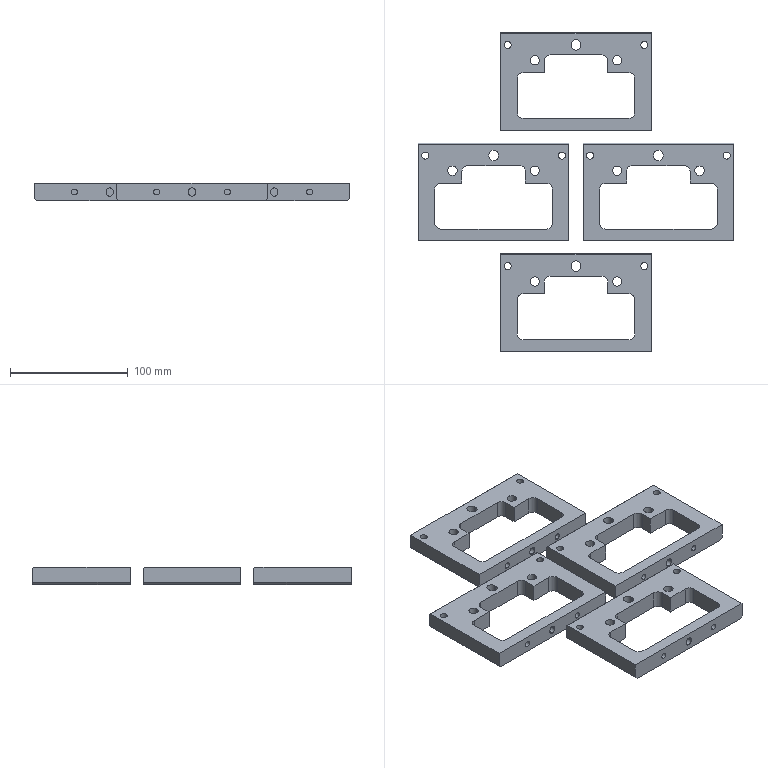NC program | NX | posted with a generic post | part box 268 x 271 x 15 mm
Lines 30 to 910 of 2286:
(ZLEVEL_PROFILE_COPY_COPY , TOOL : D4)
N52 T04 M6
N54 G54
N56 G17 G0 G90 X0.237 Y1.368 B0. C0. S9500 M3
N58 G43 Z30. H4
N60 Z1.5
N62 G94 G1 X0.139 Y1.399 Z1.495 F1000.
N64 X-0.131 Y1.401 Z1.48
N66 X-0.407 Y1.314 Z1.465
N68 X-0.642 Y1.145 Z1.45
N70 X-0.812 Y0.911 Z1.435
N72 X-0.9 Y0.635 Z1.42
N74 Y-0.612 Z1.354
N76 X-0.84 Y-0.851 Z1.342
N78 X-0.673 Y-1.113 Z1.325
N80 X-0.427 Y-1.304 Z1.309
N82 X-0.132 Y-1.4 Z1.293
N84 X0.179 Y-1.392 Z1.276
N86 X0.469 Y-1.28 Z1.26
N88 X0.677 Y-1.108 Z1.246
N90 X0.823 Y-0.888 Z1.232
N92 X0.9 Y-0.635 Z1.218
N94 Y0.635 Z1.152
N96 X0.813 Y0.909 Z1.137
N98 X0.645 Y1.142 Z1.122
N100 X0.412 Y1.311 Z1.106
N102 X0.139 Y1.399 Z1.091
N104 X-0.131 Y1.401 Z1.077
N106 X-0.407 Y1.314 Z1.062
N108 X-0.642 Y1.145 Z1.047
N110 X-0.812 Y0.911 Z1.032
N112 X-0.9 Y0.635 Z1.017
N114 Y-0.612 Z0.951
N116 X-0.84 Y-0.851 Z0.938
N118 X-0.673 Y-1.113 Z0.922
N120 X-0.427 Y-1.304 Z0.906
N122 X-0.132 Y-1.4 Z0.889
N124 X0.179 Y-1.392 Z0.873
N126 X0.469 Y-1.28 Z0.857
N128 X0.677 Y-1.108 Z0.843
N130 X0.823 Y-0.888 Z0.829
N132 X0.9 Y-0.635 Z0.815
N134 Y0.635 Z0.749
N136 X0.813 Y0.909 Z0.733
N138 X0.645 Y1.142 Z0.718
N140 X0.412 Y1.311 Z0.703
N142 X0.139 Y1.399 Z0.688
N144 X-0.131 Y1.401 Z0.674
N146 X-0.407 Y1.314 Z0.659
N148 X-0.642 Y1.145 Z0.644
N150 X-0.812 Y0.911 Z0.629
N152 X-0.9 Y0.635 Z0.613
N154 Y-0.612 Z0.548
N156 X-0.84 Y-0.851 Z0.535
N158 X-0.673 Y-1.113 Z0.519
N160 X-0.427 Y-1.304 Z0.503
N162 X-0.132 Y-1.4 Z0.486
N164 X0.179 Y-1.392 Z0.47
N166 X0.469 Y-1.28 Z0.454
N168 X0.677 Y-1.108 Z0.44
N170 X0.823 Y-0.888 Z0.426
N172 X0.9 Y-0.635 Z0.412
N174 Y0.635 Z0.345
N176 X0.813 Y0.909 Z0.33
N178 X0.645 Y1.142 Z0.315
N180 X0.412 Y1.311 Z0.3
N182 X0.139 Y1.399 Z0.285
N184 X-0.131 Y1.401 Z0.271
N186 X-0.407 Y1.314 Z0.256
N188 X-0.642 Y1.145 Z0.241
N190 X-0.812 Y0.911 Z0.225
N192 X-0.9 Y0.635 Z0.21
N194 Y-0.612 Z0.145
N196 X-0.84 Y-0.851 Z0.132
N198 X-0.673 Y-1.113 Z0.116
N200 X-0.427 Y-1.304 Z0.099
N202 X-0.132 Y-1.4 Z0.083
N204 X0.179 Y-1.392 Z0.067
N206 X0.469 Y-1.28 Z0.051
N208 X0.677 Y-1.108 Z0.036
N210 X0.823 Y-0.888 Z0.023
N212 X0.9 Y-0.635 Z0.009
N214 Y0.635 Z-0.058
N216 X0.813 Y0.909 Z-0.073
N218 X0.645 Y1.142 Z-0.088
N220 X0.412 Y1.311 Z-0.103
N222 X0.139 Y1.399 Z-0.118
N224 X-0.131 Y1.401 Z-0.132
N226 X-0.407 Y1.314 Z-0.147
N228 X-0.642 Y1.145 Z-0.163
N230 X-0.812 Y0.911 Z-0.178
N232 X-0.9 Y0.635 Z-0.193
N234 Y0.5 Z-0.2
N236 Y-0.5 F1200.
N238 G3 X0. Y-1.4 R0.9
N240 X0.9 Y-0.5 R0.9
N242 G1 Y0.5
N244 G3 X0. Y1.4 R0.9
N246 X-0.9 Y0.5 R0.9
N248 G1 Y-0.361 Z-0.23
N250 X-0.887 Y-0.589 Z-0.238
N252 X-0.881 Y-0.646 Z-0.24
N254 X-0.856 Y-0.754 Z-0.244
N256 X-0.838 Y-0.806 Z-0.246
N258 X-0.823 Y-0.843 Z-0.247
N260 X-0.791 Y-0.915 Z-0.25
N262 X-0.733 Y-1.009 Z-0.254
N264 X-0.7 Y-1.052 Z-0.256
N266 X-0.674 Y-1.083 Z-0.257
N268 X-0.62 Y-1.142 Z-0.26
N270 X-0.535 Y-1.215 Z-0.264
N272 X-0.456 Y-1.266 Z-0.267
N274 X-0.388 Y-1.304 Z-0.27
N276 X-0.285 Y-1.347 Z-0.274
N278 X-0.193 Y-1.37 Z-0.277
N280 X-0.116 Y-1.385 Z-0.28
N282 X-0.002 Y-1.394 Z-0.284
N284 X0.092 Y-1.387 Z-0.287
N286 X0.167 Y-1.376 Z-0.29
N288 X0.278 Y-1.349 Z-0.294
N290 X0.366 Y-1.313 Z-0.297
N292 X0.434 Y-1.28 Z-0.3
N294 X0.53 Y-1.219 Z-0.304
N296 X0.602 Y-1.158 Z-0.307
N298 X0.656 Y-1.104 Z-0.31
N300 X0.73 Y-1.015 Z-0.314
N302 X0.779 Y-0.934 Z-0.317
N304 X0.812 Y-0.868 Z-0.32
N306 X0.851 Y-0.775 Z-0.324
N308 X0.873 Y-0.683 Z-0.327
N310 X0.887 Y-0.595 Z-0.33
N312 X0.897 Y-0.452 Z-0.335
N314 X0.9 Y-0.309 Z-0.34
N316 Y0.265 Z-0.36
N318 Y0.409 Z-0.365
N320 X0.89 Y0.552 Z-0.37
N322 X0.873 Y0.681 Z-0.375
N324 X0.851 Y0.773 Z-0.378
N326 X0.828 Y0.828 Z-0.38
N328 X0.775 Y0.942 Z-0.384
N330 X0.725 Y1.023 Z-0.388
N332 X0.684 Y1.072 Z-0.39
N334 X0.584 Y1.173 Z-0.395
N336 X0.475 Y1.265 Z-0.4
N338 G3 X-0.9 Y0.5 R0.9
N340 G1 Y-0.361 Z-0.43
N342 X-0.887 Y-0.589 Z-0.438
N344 X-0.881 Y-0.646 Z-0.44
N346 X-0.856 Y-0.754 Z-0.444
N348 X-0.838 Y-0.806 Z-0.446
N350 X-0.823 Y-0.843 Z-0.447
N352 X-0.791 Y-0.915 Z-0.45
N354 X-0.733 Y-1.009 Z-0.454
N356 X-0.7 Y-1.052 Z-0.456
N358 X-0.674 Y-1.083 Z-0.457
N360 X-0.62 Y-1.142 Z-0.46
N362 X-0.535 Y-1.215 Z-0.464
N364 X-0.456 Y-1.266 Z-0.467
N366 X-0.388 Y-1.304 Z-0.47
N368 X-0.285 Y-1.347 Z-0.474
N370 X-0.193 Y-1.37 Z-0.477
N372 X-0.116 Y-1.385 Z-0.48
N374 X-0.002 Y-1.394 Z-0.484
N376 X0.092 Y-1.387 Z-0.487
N378 X0.167 Y-1.376 Z-0.49
N380 X0.278 Y-1.349 Z-0.494
N382 X0.366 Y-1.313 Z-0.497
N384 X0.434 Y-1.28 Z-0.5
N386 X0.53 Y-1.219 Z-0.504
N388 X0.602 Y-1.158 Z-0.507
N390 X0.656 Y-1.104 Z-0.51
N392 X0.73 Y-1.015 Z-0.514
N394 X0.779 Y-0.934 Z-0.517
N396 X0.812 Y-0.868 Z-0.52
N398 X0.85 Y-0.775 Z-0.524
N400 X0.873 Y-0.683 Z-0.527
N402 X0.887 Y-0.595 Z-0.53
N404 X0.897 Y-0.452 Z-0.535
N406 X0.9 Y-0.309 Z-0.54
N408 Y0.265 Z-0.56
N410 Y0.409 Z-0.565
N412 X0.89 Y0.552 Z-0.57
N414 X0.873 Y0.682 Z-0.575
N416 X0.851 Y0.773 Z-0.578
N418 X0.828 Y0.828 Z-0.58
N420 X0.775 Y0.942 Z-0.584
N422 X0.725 Y1.023 Z-0.588
N424 X0.684 Y1.072 Z-0.59
N426 X0.584 Y1.173 Z-0.595
N428 X0.475 Y1.265 Z-0.6
N430 G3 X-0.9 Y0.5 R0.9
N432 G1 Y-0.361 Z-0.63
N434 X-0.887 Y-0.589 Z-0.638
N436 X-0.881 Y-0.646 Z-0.64
N438 X-0.856 Y-0.754 Z-0.644
N440 X-0.838 Y-0.806 Z-0.646
N442 X-0.823 Y-0.843 Z-0.647
N444 X-0.791 Y-0.915 Z-0.65
N446 X-0.733 Y-1.009 Z-0.654
N448 X-0.701 Y-1.052 Z-0.656
N450 X-0.674 Y-1.083 Z-0.657
N452 X-0.62 Y-1.142 Z-0.66
N454 X-0.535 Y-1.215 Z-0.664
N456 X-0.456 Y-1.266 Z-0.667
N458 X-0.388 Y-1.304 Z-0.67
N460 X-0.285 Y-1.347 Z-0.674
N462 X-0.193 Y-1.37 Z-0.677
N464 X-0.116 Y-1.385 Z-0.68
N466 X-0.002 Y-1.394 Z-0.684
N468 X0.092 Y-1.387 Z-0.687
N470 X0.167 Y-1.376 Z-0.69
N472 X0.278 Y-1.349 Z-0.694
N474 X0.366 Y-1.313 Z-0.697
N476 X0.434 Y-1.28 Z-0.7
N478 X0.53 Y-1.219 Z-0.704
N480 X0.601 Y-1.158 Z-0.707
N482 X0.656 Y-1.104 Z-0.71
N484 X0.73 Y-1.015 Z-0.714
N486 X0.779 Y-0.934 Z-0.717
N488 X0.812 Y-0.868 Z-0.72
N490 X0.85 Y-0.775 Z-0.724
N492 X0.873 Y-0.683 Z-0.727
N494 X0.887 Y-0.595 Z-0.73
N496 X0.897 Y-0.452 Z-0.735
N498 X0.9 Y-0.309 Z-0.74
N500 Y0.265 Z-0.76
N502 Y0.409 Z-0.765
N504 X0.89 Y0.552 Z-0.77
N506 X0.873 Y0.682 Z-0.775
N508 X0.851 Y0.773 Z-0.778
N510 X0.828 Y0.828 Z-0.78
N512 X0.775 Y0.942 Z-0.784
N514 X0.725 Y1.022 Z-0.788
N516 X0.684 Y1.072 Z-0.79
N518 X0.584 Y1.173 Z-0.795
N520 X0.475 Y1.265 Z-0.8
N522 G3 X-0.9 Y0.5 R0.9
N524 G1 Y-0.361 Z-0.83
N526 X-0.887 Y-0.589 Z-0.838
N528 X-0.881 Y-0.646 Z-0.84
N530 X-0.856 Y-0.754 Z-0.844
N532 X-0.838 Y-0.806 Z-0.846
N534 X-0.823 Y-0.843 Z-0.847
N536 X-0.791 Y-0.915 Z-0.85
N538 X-0.733 Y-1.009 Z-0.854
N540 X-0.701 Y-1.052 Z-0.856
N542 X-0.675 Y-1.083 Z-0.857
N544 X-0.62 Y-1.142 Z-0.86
N546 X-0.535 Y-1.215 Z-0.864
N548 X-0.456 Y-1.266 Z-0.867
N550 X-0.388 Y-1.304 Z-0.87
N552 X-0.285 Y-1.347 Z-0.874
N554 X-0.193 Y-1.37 Z-0.877
N556 X-0.116 Y-1.385 Z-0.88
N558 X-0.003 Y-1.394 Z-0.884
N560 X0.092 Y-1.387 Z-0.887
N562 X0.167 Y-1.376 Z-0.89
N564 X0.278 Y-1.349 Z-0.894
N566 X0.365 Y-1.313 Z-0.897
N568 X0.434 Y-1.28 Z-0.9
N570 X0.53 Y-1.219 Z-0.904
N572 X0.601 Y-1.158 Z-0.907
N574 X0.656 Y-1.104 Z-0.91
N576 X0.729 Y-1.015 Z-0.914
N578 X0.779 Y-0.934 Z-0.917
N580 X0.812 Y-0.868 Z-0.92
N582 X0.85 Y-0.775 Z-0.924
N584 X0.873 Y-0.684 Z-0.927
N586 X0.887 Y-0.595 Z-0.93
N588 X0.897 Y-0.452 Z-0.935
N590 X0.9 Y-0.309 Z-0.94
N592 Y0.265 Z-0.96
N594 Y0.409 Z-0.965
N596 X0.89 Y0.552 Z-0.97
N598 X0.873 Y0.682 Z-0.975
N600 X0.851 Y0.773 Z-0.978
N602 X0.828 Y0.828 Z-0.98
N604 X0.775 Y0.942 Z-0.984
N606 X0.725 Y1.022 Z-0.988
N608 X0.684 Y1.072 Z-0.99
N610 X0.584 Y1.173 Z-0.995
N612 X0.475 Y1.265 Z-1.
N614 G3 X-0.9 Y0.5 R0.9
N616 G1 Y-0.361 Z-1.03
N618 X-0.887 Y-0.588 Z-1.038
N620 X-0.881 Y-0.646 Z-1.04
N622 X-0.856 Y-0.754 Z-1.044
N624 X-0.838 Y-0.806 Z-1.046
N626 X-0.823 Y-0.843 Z-1.047
N628 X-0.791 Y-0.915 Z-1.05
N630 X-0.733 Y-1.009 Z-1.054
N632 X-0.701 Y-1.052 Z-1.056
N634 X-0.675 Y-1.083 Z-1.057
N636 X-0.62 Y-1.142 Z-1.06
N638 X-0.535 Y-1.215 Z-1.064
N640 X-0.456 Y-1.266 Z-1.067
N642 X-0.388 Y-1.304 Z-1.07
N644 X-0.285 Y-1.347 Z-1.074
N646 X-0.193 Y-1.37 Z-1.077
N648 X-0.116 Y-1.385 Z-1.08
N650 X-0.003 Y-1.393 Z-1.084
N652 X0.092 Y-1.387 Z-1.087
N654 X0.167 Y-1.376 Z-1.09
N656 X0.278 Y-1.35 Z-1.094
N658 X0.365 Y-1.313 Z-1.097
N660 X0.434 Y-1.28 Z-1.1
N662 X0.53 Y-1.219 Z-1.104
N664 X0.602 Y-1.158 Z-1.107
N666 X0.656 Y-1.104 Z-1.11
N668 X0.73 Y-1.014 Z-1.114
N670 X0.78 Y-0.933 Z-1.117
N672 X0.812 Y-0.868 Z-1.12
N674 X0.85 Y-0.775 Z-1.124
N676 X0.873 Y-0.683 Z-1.127
N678 X0.887 Y-0.595 Z-1.13
N680 X0.897 Y-0.452 Z-1.135
N682 X0.9 Y-0.309 Z-1.14
N684 Y0.265 Z-1.16
N686 Y0.409 Z-1.165
N688 X0.89 Y0.552 Z-1.17
N690 X0.873 Y0.682 Z-1.175
N692 X0.851 Y0.773 Z-1.178
N694 X0.828 Y0.828 Z-1.18
N696 X0.775 Y0.942 Z-1.184
N698 X0.725 Y1.022 Z-1.188
N700 X0.684 Y1.071 Z-1.19
N702 X0.584 Y1.173 Z-1.195
N704 X0.475 Y1.265 Z-1.2
N706 G3 X-0.9 Y0.5 R0.9
N708 G1 Y-0.361 Z-1.23
N710 X-0.887 Y-0.588 Z-1.238
N712 X-0.881 Y-0.646 Z-1.24
N714 X-0.856 Y-0.754 Z-1.244
N716 X-0.838 Y-0.806 Z-1.246
N718 X-0.823 Y-0.842 Z-1.247
N720 X-0.791 Y-0.915 Z-1.25
N722 X-0.733 Y-1.008 Z-1.254
N724 X-0.701 Y-1.052 Z-1.256
N726 X-0.675 Y-1.082 Z-1.257
N728 X-0.62 Y-1.142 Z-1.26
N730 X-0.535 Y-1.215 Z-1.264
N732 X-0.456 Y-1.266 Z-1.267
N734 X-0.388 Y-1.304 Z-1.27
N736 X-0.285 Y-1.347 Z-1.274
N738 X-0.193 Y-1.37 Z-1.277
N740 X-0.116 Y-1.385 Z-1.28
N742 X-0.003 Y-1.393 Z-1.284
N744 X0.091 Y-1.387 Z-1.287
N746 X0.167 Y-1.376 Z-1.29
N748 X0.278 Y-1.35 Z-1.294
N750 X0.365 Y-1.313 Z-1.297
N752 X0.434 Y-1.28 Z-1.3
N754 X0.529 Y-1.219 Z-1.304
N756 X0.602 Y-1.158 Z-1.307
N758 X0.656 Y-1.104 Z-1.31
N760 X0.73 Y-1.014 Z-1.314
N762 X0.78 Y-0.933 Z-1.317
N764 X0.812 Y-0.868 Z-1.32
N766 X0.85 Y-0.775 Z-1.324
N768 X0.873 Y-0.683 Z-1.327
N770 X0.887 Y-0.595 Z-1.33
N772 X0.897 Y-0.452 Z-1.335
N774 X0.9 Y-0.309 Z-1.34
N776 Y0.265 Z-1.36
N778 Y0.409 Z-1.365
N780 X0.89 Y0.552 Z-1.37
N782 X0.873 Y0.682 Z-1.375
N784 X0.851 Y0.773 Z-1.378
N786 X0.828 Y0.828 Z-1.38
N788 X0.775 Y0.942 Z-1.384
N790 X0.725 Y1.022 Z-1.388
N792 X0.684 Y1.071 Z-1.39
N794 X0.584 Y1.173 Z-1.395
N796 X0.475 Y1.265 Z-1.4
N798 G3 X-0.9 Y0.5 R0.9
N800 G1 Y-0.361 Z-1.43
N802 X-0.887 Y-0.588 Z-1.438
N804 X-0.881 Y-0.646 Z-1.44
N806 X-0.856 Y-0.754 Z-1.444
N808 X-0.838 Y-0.806 Z-1.446
N810 X-0.823 Y-0.842 Z-1.447
N812 X-0.791 Y-0.915 Z-1.45
N814 X-0.733 Y-1.008 Z-1.454
N816 X-0.701 Y-1.052 Z-1.456
N818 X-0.675 Y-1.082 Z-1.457
N820 X-0.62 Y-1.142 Z-1.46
N822 X-0.535 Y-1.215 Z-1.464
N824 X-0.456 Y-1.266 Z-1.467
N826 X-0.388 Y-1.304 Z-1.47
N828 X-0.285 Y-1.347 Z-1.474
N830 X-0.193 Y-1.37 Z-1.477
N832 X-0.116 Y-1.385 Z-1.48
N834 X-0.003 Y-1.393 Z-1.484
N836 X0.091 Y-1.387 Z-1.487
N838 X0.167 Y-1.376 Z-1.49
N840 X0.278 Y-1.35 Z-1.494
N842 X0.365 Y-1.313 Z-1.497
N844 X0.434 Y-1.28 Z-1.5
N846 X0.531 Y-1.218 Z-1.504
N848 X0.603 Y-1.158 Z-1.507
N850 X0.656 Y-1.104 Z-1.51
N852 X0.73 Y-1.013 Z-1.514
N854 X0.78 Y-0.933 Z-1.517
N856 X0.812 Y-0.868 Z-1.52
N858 X0.85 Y-0.775 Z-1.524
N860 X0.873 Y-0.683 Z-1.527
N862 X0.887 Y-0.595 Z-1.53
N864 X0.897 Y-0.452 Z-1.535
N866 X0.9 Y-0.309 Z-1.54
N868 Y0.265 Z-1.56
N870 Y0.409 Z-1.565
N872 X0.889 Y0.552 Z-1.57
N874 X0.873 Y0.682 Z-1.575
N876 X0.851 Y0.773 Z-1.578
N878 X0.828 Y0.828 Z-1.58
N880 X0.775 Y0.942 Z-1.584
N882 X0.725 Y1.022 Z-1.588
N884 X0.684 Y1.071 Z-1.59
N886 X0.584 Y1.173 Z-1.595
N888 X0.475 Y1.265 Z-1.6
N890 G3 X-0.9 Y0.5 R0.9
N892 G1 Y-0.361 Z-1.63
N894 X-0.887 Y-0.588 Z-1.638
N896 X-0.881 Y-0.646 Z-1.64
N898 X-0.856 Y-0.754 Z-1.644
N900 X-0.838 Y-0.806 Z-1.646
N902 X-0.823 Y-0.842 Z-1.647
N904 X-0.791 Y-0.915 Z-1.65
N906 X-0.733 Y-1.008 Z-1.654
N908 X-0.701 Y-1.052 Z-1.656
N910 X-0.675 Y-1.082 Z-1.657
N912 X-0.62 Y-1.142 Z-1.66
N914 X-0.535 Y-1.215 Z-1.664
N916 X-0.456 Y-1.266 Z-1.667
N918 X-0.388 Y-1.304 Z-1.67
N920 X-0.285 Y-1.347 Z-1.674
N922 X-0.193 Y-1.37 Z-1.677
N924 X-0.116 Y-1.385 Z-1.68
N926 X-0.003 Y-1.394 Z-1.684
N928 X0.091 Y-1.386 Z-1.687
N930 X0.167 Y-1.376 Z-1.69
N932 X0.278 Y-1.35 Z-1.694
N934 X0.365 Y-1.313 Z-1.697
N936 X0.434 Y-1.28 Z-1.7
N938 X0.53 Y-1.219 Z-1.704
N940 X0.603 Y-1.158 Z-1.707
N942 X0.656 Y-1.104 Z-1.71
N944 X0.73 Y-1.013 Z-1.714
N946 X0.78 Y-0.933 Z-1.717
N948 X0.812 Y-0.868 Z-1.72
N950 X0.85 Y-0.775 Z-1.724
N952 X0.872 Y-0.683 Z-1.727
N954 X0.887 Y-0.595 Z-1.73
N956 X0.897 Y-0.452 Z-1.735
N958 X0.9 Y-0.309 Z-1.74
N960 Y0.265 Z-1.76
N962 Y0.409 Z-1.765
N964 X0.889 Y0.552 Z-1.77
N966 X0.873 Y0.682 Z-1.775
N968 X0.851 Y0.773 Z-1.778
N970 X0.828 Y0.828 Z-1.78
N972 X0.775 Y0.942 Z-1.784
N974 X0.725 Y1.022 Z-1.788
N976 X0.684 Y1.071 Z-1.79
N978 X0.584 Y1.173 Z-1.795
N980 X0.475 Y1.265 Z-1.8
N982 G3 X-0.9 Y0.5 R0.9
N984 G1 Y-0.361 Z-1.83
N986 X-0.887 Y-0.588 Z-1.838
N988 X-0.881 Y-0.646 Z-1.84
N990 X-0.856 Y-0.754 Z-1.844
N992 X-0.838 Y-0.806 Z-1.846
N994 X-0.823 Y-0.842 Z-1.847
N996 X-0.791 Y-0.915 Z-1.85
N998 X-0.733 Y-1.008 Z-1.854
N1000 X-0.701 Y-1.052 Z-1.856
N1002 X-0.675 Y-1.082 Z-1.857
N1004 X-0.62 Y-1.142 Z-1.86
N1006 X-0.535 Y-1.215 Z-1.864
N1008 X-0.456 Y-1.266 Z-1.867
N1010 X-0.388 Y-1.304 Z-1.87
N1012 X-0.285 Y-1.347 Z-1.874
N1014 X-0.194 Y-1.37 Z-1.877
N1016 X-0.116 Y-1.385 Z-1.88
N1018 X-0.003 Y-1.394 Z-1.884
N1020 X0.091 Y-1.386 Z-1.887
N1022 X0.167 Y-1.376 Z-1.89
N1024 X0.278 Y-1.35 Z-1.894
N1026 X0.365 Y-1.313 Z-1.897
N1028 X0.434 Y-1.28 Z-1.9
N1030 X0.531 Y-1.219 Z-1.904
N1032 X0.602 Y-1.158 Z-1.907
N1034 X0.656 Y-1.104 Z-1.91
N1036 X0.73 Y-1.013 Z-1.914
N1038 X0.78 Y-0.933 Z-1.917
N1040 X0.812 Y-0.868 Z-1.92
N1042 X0.85 Y-0.775 Z-1.924
N1044 X0.872 Y-0.683 Z-1.927
N1046 X0.887 Y-0.595 Z-1.93
N1048 X0.897 Y-0.452 Z-1.935
N1050 X0.9 Y-0.309 Z-1.94
N1052 Y0.265 Z-1.96
N1054 Y0.409 Z-1.965
N1056 X0.889 Y0.552 Z-1.97
N1058 X0.873 Y0.682 Z-1.975
N1060 X0.851 Y0.773 Z-1.978
N1062 X0.828 Y0.828 Z-1.98
N1064 X0.775 Y0.942 Z-1.984
N1066 X0.725 Y1.022 Z-1.988
N1068 X0.684 Y1.071 Z-1.99
N1070 X0.584 Y1.173 Z-1.995
N1072 X0.475 Y1.265 Z-2.
N1074 G3 X-0.9 Y0.5 R0.9
N1076 G1 Y-0.361 Z-2.03
N1078 X-0.887 Y-0.588 Z-2.038
N1080 X-0.881 Y-0.646 Z-2.04
N1082 X-0.856 Y-0.754 Z-2.044
N1084 X-0.838 Y-0.806 Z-2.046
N1086 X-0.823 Y-0.842 Z-2.047
N1088 X-0.791 Y-0.915 Z-2.05
N1090 X-0.734 Y-1.009 Z-2.054
N1092 X-0.701 Y-1.052 Z-2.056
N1094 X-0.675 Y-1.082 Z-2.057
N1096 X-0.62 Y-1.142 Z-2.06
N1098 X-0.535 Y-1.215 Z-2.064
N1100 X-0.456 Y-1.266 Z-2.067
N1102 X-0.388 Y-1.304 Z-2.07
N1104 X-0.285 Y-1.346 Z-2.074
N1106 X-0.194 Y-1.37 Z-2.077
N1108 X-0.116 Y-1.385 Z-2.08
N1110 X-0.003 Y-1.394 Z-2.084
N1112 X0.091 Y-1.386 Z-2.087
N1114 X0.167 Y-1.376 Z-2.09
N1116 X0.278 Y-1.35 Z-2.094
N1118 X0.365 Y-1.313 Z-2.097
N1120 X0.434 Y-1.28 Z-2.1
N1122 X0.531 Y-1.219 Z-2.104
N1124 X0.602 Y-1.158 Z-2.107
N1126 X0.656 Y-1.104 Z-2.11
N1128 X0.731 Y-1.014 Z-2.114
N1130 X0.78 Y-0.933 Z-2.117
N1132 X0.812 Y-0.868 Z-2.12
N1134 X0.85 Y-0.775 Z-2.124
N1136 X0.872 Y-0.683 Z-2.127
N1138 X0.886 Y-0.595 Z-2.13
N1140 X0.897 Y-0.452 Z-2.135
N1142 X0.9 Y-0.309 Z-2.14
N1144 Y0.265 Z-2.16
N1146 Y0.409 Z-2.165
N1148 X0.889 Y0.552 Z-2.17
N1150 X0.873 Y0.682 Z-2.175
N1152 X0.851 Y0.773 Z-2.178
N1154 X0.828 Y0.828 Z-2.18
N1156 X0.775 Y0.941 Z-2.184
N1158 X0.725 Y1.022 Z-2.188
N1160 X0.684 Y1.071 Z-2.19
N1162 X0.584 Y1.173 Z-2.195
N1164 X0.475 Y1.265 Z-2.2
N1166 G3 X-0.9 Y0.5 R0.9
N1168 G1 Y-0.361 Z-2.23
N1170 X-0.886 Y-0.588 Z-2.238
N1172 X-0.881 Y-0.646 Z-2.24
N1174 X-0.856 Y-0.754 Z-2.244
N1176 X-0.838 Y-0.805 Z-2.246
N1178 X-0.823 Y-0.842 Z-2.247
N1180 X-0.791 Y-0.915 Z-2.25
N1182 X-0.734 Y-1.008 Z-2.254
N1184 X-0.701 Y-1.051 Z-2.256
N1186 X-0.675 Y-1.082 Z-2.257
N1188 X-0.62 Y-1.142 Z-2.26
N1190 X-0.535 Y-1.214 Z-2.264
N1192 X-0.456 Y-1.266 Z-2.267
N1194 X-0.388 Y-1.304 Z-2.27
N1196 X-0.285 Y-1.346 Z-2.274
N1198 X-0.194 Y-1.37 Z-2.277
N1200 X-0.116 Y-1.385 Z-2.28
N1202 X-0.003 Y-1.394 Z-2.284
N1204 X0.091 Y-1.386 Z-2.287
N1206 X0.167 Y-1.376 Z-2.29
N1208 X0.278 Y-1.349 Z-2.294
N1210 X0.365 Y-1.313 Z-2.297
N1212 X0.434 Y-1.28 Z-2.3
N1214 X0.531 Y-1.219 Z-2.304
N1216 X0.602 Y-1.158 Z-2.307
N1218 X0.656 Y-1.104 Z-2.31
N1220 X0.73 Y-1.014 Z-2.314
N1222 X0.779 Y-0.933 Z-2.317
N1224 X0.812 Y-0.868 Z-2.32
N1226 X0.85 Y-0.775 Z-2.324
N1228 X0.872 Y-0.684 Z-2.327
N1230 X0.886 Y-0.595 Z-2.33
N1232 X0.897 Y-0.452 Z-2.335
N1234 X0.9 Y-0.309 Z-2.34
N1236 Y0.265 Z-2.36
N1238 Y0.409 Z-2.365
N1240 X0.889 Y0.552 Z-2.37
N1242 X0.873 Y0.682 Z-2.375
N1244 X0.851 Y0.773 Z-2.378
N1246 X0.828 Y0.828 Z-2.38
N1248 X0.775 Y0.941 Z-2.384
N1250 X0.725 Y1.022 Z-2.388
N1252 X0.684 Y1.071 Z-2.39
N1254 X0.583 Y1.173 Z-2.395
N1256 X0.475 Y1.265 Z-2.4
N1258 G3 X-0.9 Y0.5 R0.9
N1260 G1 Y-0.361 Z-2.43
N1262 X-0.886 Y-0.588 Z-2.438
N1264 X-0.881 Y-0.646 Z-2.44
N1266 X-0.856 Y-0.753 Z-2.444
N1268 X-0.838 Y-0.805 Z-2.446
N1270 X-0.823 Y-0.842 Z-2.447
N1272 X-0.791 Y-0.915 Z-2.45
N1274 X-0.734 Y-1.008 Z-2.454
N1276 X-0.701 Y-1.051 Z-2.456
N1278 X-0.675 Y-1.082 Z-2.457
N1280 X-0.62 Y-1.142 Z-2.46
N1282 X-0.535 Y-1.214 Z-2.464
N1284 X-0.456 Y-1.266 Z-2.467
N1286 X-0.388 Y-1.304 Z-2.47
N1288 X-0.285 Y-1.346 Z-2.474
N1290 X-0.194 Y-1.37 Z-2.477
N1292 X-0.116 Y-1.384 Z-2.48
N1294 X-0.003 Y-1.394 Z-2.484
N1296 X0.091 Y-1.387 Z-2.487
N1298 X0.167 Y-1.376 Z-2.49
N1300 X0.279 Y-1.349 Z-2.494
N1302 X0.366 Y-1.313 Z-2.497
N1304 X0.434 Y-1.28 Z-2.5
N1306 X0.531 Y-1.219 Z-2.504
N1308 X0.602 Y-1.157 Z-2.507
N1310 X0.656 Y-1.104 Z-2.51
N1312 X0.73 Y-1.014 Z-2.514
N1314 X0.779 Y-0.933 Z-2.517
N1316 X0.812 Y-0.868 Z-2.52
N1318 X0.85 Y-0.775 Z-2.523
N1320 X0.872 Y-0.684 Z-2.527
N1322 X0.886 Y-0.595 Z-2.53
N1324 X0.897 Y-0.452 Z-2.535
N1326 X0.9 Y-0.309 Z-2.54
N1328 Y0.265 Z-2.56
N1330 Y0.409 Z-2.565
N1332 X0.889 Y0.552 Z-2.57
N1334 X0.873 Y0.682 Z-2.575
N1336 X0.851 Y0.773 Z-2.578
N1338 X0.828 Y0.828 Z-2.58
N1340 X0.775 Y0.941 Z-2.584
N1342 X0.725 Y1.022 Z-2.588
N1344 X0.684 Y1.071 Z-2.59
N1346 X0.583 Y1.173 Z-2.595
N1348 X0.475 Y1.265 Z-2.6
N1350 G3 X-0.9 Y0.5 R0.9
N1352 G1 Y-0.361 Z-2.63
N1354 X-0.886 Y-0.588 Z-2.638
N1356 X-0.881 Y-0.646 Z-2.64
N1358 X-0.856 Y-0.753 Z-2.644
N1360 X-0.838 Y-0.805 Z-2.646
N1362 X-0.823 Y-0.842 Z-2.647
N1364 X-0.791 Y-0.915 Z-2.65
N1366 X-0.734 Y-1.008 Z-2.654
N1368 X-0.701 Y-1.051 Z-2.656
N1370 X-0.675 Y-1.082 Z-2.657
N1372 X-0.62 Y-1.142 Z-2.66
N1374 X-0.535 Y-1.214 Z-2.664
N1376 X-0.456 Y-1.265 Z-2.667
N1378 X-0.388 Y-1.304 Z-2.67
N1380 X-0.285 Y-1.346 Z-2.674
N1382 X-0.194 Y-1.37 Z-2.677
N1384 X-0.116 Y-1.384 Z-2.68
N1386 X-0.003 Y-1.394 Z-2.684
N1388 X0.091 Y-1.387 Z-2.687
N1390 X0.167 Y-1.376 Z-2.69
N1392 X0.279 Y-1.349 Z-2.694
N1394 X0.366 Y-1.313 Z-2.697
N1396 X0.434 Y-1.28 Z-2.7
N1398 X0.531 Y-1.219 Z-2.704
N1400 X0.602 Y-1.157 Z-2.707
N1402 X0.656 Y-1.104 Z-2.71
N1404 X0.73 Y-1.014 Z-2.714
N1406 X0.779 Y-0.933 Z-2.717
N1408 X0.812 Y-0.868 Z-2.72
N1410 X0.85 Y-0.775 Z-2.723
N1412 X0.872 Y-0.684 Z-2.727
N1414 X0.886 Y-0.595 Z-2.73
N1416 X0.897 Y-0.452 Z-2.735
N1418 X0.9 Y-0.309 Z-2.74
N1420 Y0.265 Z-2.76
N1422 Y0.409 Z-2.765
N1424 X0.889 Y0.552 Z-2.77
N1426 X0.873 Y0.682 Z-2.775
N1428 X0.851 Y0.773 Z-2.778
N1430 X0.828 Y0.828 Z-2.78
N1432 X0.775 Y0.941 Z-2.784
N1434 X0.725 Y1.022 Z-2.788
N1436 X0.684 Y1.071 Z-2.79
N1438 X0.583 Y1.173 Z-2.795
N1440 X0.475 Y1.265 Z-2.8
N1442 G3 X-0.9 Y0.5 R0.9
N1444 G1 Y-0.361 Z-2.83
N1446 X-0.886 Y-0.588 Z-2.838
N1448 X-0.881 Y-0.646 Z-2.84
N1450 X-0.856 Y-0.753 Z-2.844
N1452 X-0.838 Y-0.805 Z-2.846
N1454 X-0.823 Y-0.842 Z-2.847
N1456 X-0.791 Y-0.915 Z-2.85
N1458 X-0.734 Y-1.008 Z-2.854
N1460 X-0.701 Y-1.051 Z-2.856
N1462 X-0.675 Y-1.082 Z-2.857
N1464 X-0.62 Y-1.142 Z-2.86
N1466 X-0.535 Y-1.214 Z-2.864
N1468 X-0.456 Y-1.265 Z-2.867
N1470 X-0.388 Y-1.304 Z-2.87
N1472 X-0.285 Y-1.346 Z-2.874
N1474 X-0.194 Y-1.37 Z-2.877
N1476 X-0.116 Y-1.384 Z-2.88
N1478 X-0.003 Y-1.394 Z-2.884
N1480 X0.091 Y-1.387 Z-2.887
N1482 X0.167 Y-1.376 Z-2.89
N1484 X0.279 Y-1.349 Z-2.894
N1486 X0.366 Y-1.313 Z-2.897
N1488 X0.434 Y-1.28 Z-2.9
N1490 X0.531 Y-1.219 Z-2.904
N1492 X0.602 Y-1.157 Z-2.907
N1494 X0.656 Y-1.104 Z-2.91
N1496 X0.73 Y-1.014 Z-2.914
N1498 X0.779 Y-0.933 Z-2.917
N1500 X0.812 Y-0.868 Z-2.92
N1502 X0.85 Y-0.776 Z-2.923
N1504 X0.872 Y-0.684 Z-2.927
N1506 X0.886 Y-0.595 Z-2.93
N1508 X0.897 Y-0.452 Z-2.935
N1510 X0.9 Y-0.309 Z-2.94
N1512 Y0.265 Z-2.96
N1514 Y0.409 Z-2.965
N1516 X0.889 Y0.552 Z-2.97
N1518 X0.873 Y0.682 Z-2.975
N1520 X0.851 Y0.774 Z-2.978
N1522 X0.828 Y0.828 Z-2.98
N1524 X0.775 Y0.941 Z-2.984
N1526 X0.725 Y1.022 Z-2.988
N1528 X0.684 Y1.071 Z-2.99
N1530 X0.583 Y1.173 Z-2.995
N1532 X0.475 Y1.265 Z-3.
N1534 G3 X-0.9 Y0.5 R0.9
N1536 G1 Y-0.361 Z-3.03
N1538 X-0.886 Y-0.588 Z-3.038
N1540 X-0.881 Y-0.646 Z-3.04
N1542 X-0.855 Y-0.753 Z-3.044
N1544 X-0.838 Y-0.805 Z-3.046
N1546 X-0.823 Y-0.842 Z-3.047
N1548 X-0.791 Y-0.915 Z-3.05
N1550 X-0.734 Y-1.008 Z-3.054
N1552 X-0.701 Y-1.051 Z-3.056
N1554 X-0.675 Y-1.082 Z-3.057
N1556 X-0.62 Y-1.142 Z-3.06
N1558 X-0.535 Y-1.214 Z-3.064
N1560 X-0.456 Y-1.265 Z-3.067
N1562 X-0.388 Y-1.304 Z-3.07
N1564 X-0.285 Y-1.346 Z-3.074
N1566 X-0.194 Y-1.37 Z-3.077
N1568 X-0.116 Y-1.384 Z-3.08
N1570 X-0.003 Y-1.394 Z-3.084
N1572 X0.091 Y-1.387 Z-3.087
N1574 X0.167 Y-1.376 Z-3.09
N1576 X0.279 Y-1.349 Z-3.094
N1578 X0.366 Y-1.313 Z-3.097
N1580 X0.434 Y-1.28 Z-3.1
N1582 X0.531 Y-1.219 Z-3.104
N1584 X0.602 Y-1.157 Z-3.107
N1586 X0.656 Y-1.104 Z-3.11
N1588 X0.73 Y-1.014 Z-3.114
N1590 X0.779 Y-0.933 Z-3.117
N1592 X0.812 Y-0.868 Z-3.12
N1594 X0.85 Y-0.776 Z-3.123
N1596 X0.872 Y-0.684 Z-3.127
N1598 X0.886 Y-0.595 Z-3.13
N1600 X0.897 Y-0.452 Z-3.135
N1602 X0.9 Y-0.309 Z-3.14
N1604 Y0.265 Z-3.16
N1606 Y0.409 Z-3.165
N1608 X0.889 Y0.552 Z-3.17
N1610 X0.873 Y0.682 Z-3.175
N1612 X0.85 Y0.774 Z-3.178
N1614 X0.828 Y0.828 Z-3.18
N1616 X0.775 Y0.941 Z-3.184
N1618 X0.725 Y1.021 Z-3.188
N1620 X0.683 Y1.071 Z-3.19
N1622 X0.583 Y1.173 Z-3.195
N1624 X0.475 Y1.265 Z-3.2
N1626 G3 X-0.9 Y0.5 R0.9
N1628 G1 Y-0.361 Z-3.23
N1630 X-0.886 Y-0.588 Z-3.238
N1632 X-0.881 Y-0.646 Z-3.24
N1634 X-0.855 Y-0.753 Z-3.244
N1636 X-0.838 Y-0.805 Z-3.246
N1638 X-0.823 Y-0.842 Z-3.247
N1640 X-0.791 Y-0.915 Z-3.25
N1642 X-0.734 Y-1.008 Z-3.254
N1644 X-0.701 Y-1.051 Z-3.256
N1646 X-0.675 Y-1.082 Z-3.257
N1648 X-0.62 Y-1.142 Z-3.26
N1650 X-0.535 Y-1.214 Z-3.264
N1652 X-0.456 Y-1.265 Z-3.267
N1654 X-0.388 Y-1.304 Z-3.27
N1656 X-0.285 Y-1.346 Z-3.274
N1658 X-0.194 Y-1.369 Z-3.277
N1660 X-0.116 Y-1.384 Z-3.28
N1662 X-0.003 Y-1.394 Z-3.284
N1664 X0.091 Y-1.387 Z-3.287
N1666 X0.167 Y-1.376 Z-3.29
N1668 X0.279 Y-1.349 Z-3.294
N1670 X0.366 Y-1.313 Z-3.297
N1672 X0.434 Y-1.279 Z-3.3
N1674 X0.53 Y-1.219 Z-3.304
N1676 X0.602 Y-1.157 Z-3.307
N1678 X0.656 Y-1.104 Z-3.31
N1680 X0.73 Y-1.014 Z-3.314
N1682 X0.779 Y-0.933 Z-3.317
N1684 X0.812 Y-0.868 Z-3.32
N1686 X0.85 Y-0.776 Z-3.323
N1688 X0.872 Y-0.684 Z-3.327
N1690 X0.886 Y-0.595 Z-3.33
N1692 X0.897 Y-0.452 Z-3.335
N1694 X0.9 Y-0.309 Z-3.34
N1696 Y0.265 Z-3.36
N1698 Y0.409 Z-3.365
N1700 X0.889 Y0.552 Z-3.37
N1702 X0.872 Y0.682 Z-3.375
N1704 X0.85 Y0.774 Z-3.378
N1706 X0.828 Y0.828 Z-3.38
N1708 X0.775 Y0.941 Z-3.384
N1710 X0.725 Y1.021 Z-3.388
N1712 X0.683 Y1.071 Z-3.39
N1714 X0.583 Y1.173 Z-3.395
N1716 X0.475 Y1.265 Z-3.4
N1718 G3 X-0.9 Y0.5 R0.9
N1720 G1 Y-0.361 Z-3.43
N1722 X-0.886 Y-0.588 Z-3.438
N1724 X-0.881 Y-0.646 Z-3.44
N1726 X-0.855 Y-0.753 Z-3.444
N1728 X-0.838 Y-0.805 Z-3.446
N1730 X-0.823 Y-0.842 Z-3.447
N1732 X-0.791 Y-0.915 Z-3.45
N1734 X-0.734 Y-1.008 Z-3.454
N1736 X-0.701 Y-1.051 Z-3.456
N1738 X-0.675 Y-1.082 Z-3.457
N1740 X-0.62 Y-1.142 Z-3.46
N1742 X-0.535 Y-1.214 Z-3.464
N1744 X-0.456 Y-1.265 Z-3.467
N1746 X-0.388 Y-1.304 Z-3.47
N1748 X-0.285 Y-1.346 Z-3.474
N1750 X-0.194 Y-1.369 Z-3.477
N1752 X-0.116 Y-1.384 Z-3.48
N1754 X-0.003 Y-1.394 Z-3.484
N1756 X0.091 Y-1.387 Z-3.487
N1758 X0.167 Y-1.376 Z-3.49
N1760 X0.279 Y-1.349 Z-3.494
N1762 X0.366 Y-1.313 Z-3.497
N1764 X0.434 Y-1.279 Z-3.5
N1766 X0.53 Y-1.219 Z-3.504
N1768 X0.602 Y-1.157 Z-3.507
N1770 X0.656 Y-1.104 Z-3.51
N1772 X0.73 Y-1.014 Z-3.514
N1774 X0.779 Y-0.933 Z-3.517
N1776 X0.812 Y-0.868 Z-3.52
N1778 X0.85 Y-0.776 Z-3.523
N1780 X0.872 Y-0.684 Z-3.527
N1782 X0.886 Y-0.595 Z-3.53
N1784 X0.897 Y-0.452 Z-3.535
N1786 X0.9 Y-0.309 Z-3.54
N1788 Y0.265 Z-3.56
N1790 Y0.409 Z-3.565
N1792 X0.889 Y0.552 Z-3.57
N1794 X0.872 Y0.682 Z-3.575
N1796 X0.85 Y0.774 Z-3.578
N1798 X0.828 Y0.828 Z-3.58
N1800 X0.775 Y0.941 Z-3.584
N1802 X0.725 Y1.021 Z-3.588
N1804 X0.683 Y1.071 Z-3.59
N1806 X0.583 Y1.173 Z-3.595